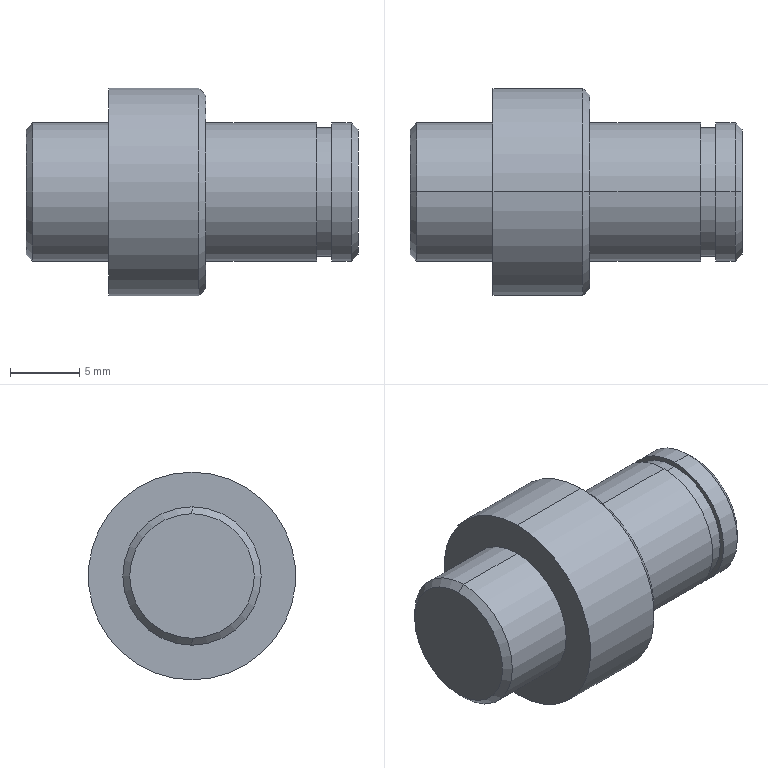Part | SolidWorks | features ICE 4, Chamfer 3, Extrusion 1, RefAxis 1 | 1 solid | 22 faces | box 24 x 15 x 15 mm | volume 2547 mm3 | cylinder 10 | cone 6 | plane 6 | commonest cylinder face diameters 10 x6 9.3 x2 15 x2
STEP:
#1=CARTESIAN_POINT('',(24.,0.,-4.5));
#2=VERTEX_POINT('',#1);
#3=CARTESIAN_POINT('',(24.,0.,4.5));
#4=VERTEX_POINT('',#3);
#5=CARTESIAN_POINT('',(24.,0.,0.));
#6=DIRECTION('',(1.,0.,0.));
#7=DIRECTION('',(0.,0.,-1.));
#8=AXIS2_PLACEMENT_3D('',#5,#6,#7);
#9=CIRCLE('',#8,4.5);
#10=EDGE_CURVE('',#2,#4,#9,.T.);
#11=ORIENTED_EDGE('',*,*,#10,.F.);
#12=CARTESIAN_POINT('',(23.5,0.,-5.));
#13=VERTEX_POINT('',#12);
#14=CARTESIAN_POINT('',(24.,0.,-4.5));
#15=DIRECTION('',(-0.7071,0.,-0.7071));
#16=VECTOR('',#15,1000.);
#17=LINE('',#14,#16);
#18=EDGE_CURVE('',#2,#13,#17,.T.);
#19=ORIENTED_EDGE('',*,*,#18,.T.);
#20=CARTESIAN_POINT('',(23.5,0.,5.));
#21=VERTEX_POINT('',#20);
#22=CARTESIAN_POINT('',(23.5,0.,0.));
#23=DIRECTION('',(-1.,0.,0.));
#24=DIRECTION('',(0.,0.,-1.));
#25=AXIS2_PLACEMENT_3D('',#22,#23,#24);
#26=CIRCLE('',#25,5.);
#27=EDGE_CURVE('',#21,#13,#26,.T.);
#28=ORIENTED_EDGE('',*,*,#27,.F.);
#29=CARTESIAN_POINT('',(24.,0.,4.5));
#30=DIRECTION('',(-0.7071,0.,0.7071));
#31=VECTOR('',#30,1000.);
#32=LINE('',#29,#31);
#33=EDGE_CURVE('',#4,#21,#32,.T.);
#34=ORIENTED_EDGE('',*,*,#33,.F.);
#35=EDGE_LOOP('',(#11,#19,#28,#34));
#36=FACE_OUTER_BOUND('',#35,.T.);
#37=CARTESIAN_POINT('',(24.,0.,0.));
#38=DIRECTION('',(-1.,0.,0.));
#39=DIRECTION('',(0.,0.,1.));
#40=AXIS2_PLACEMENT_3D('',#37,#38,#39);
#41=CONICAL_SURFACE('',#40,4.5,0.7854);
#42=ADVANCED_FACE('',(#36),#41,.T.);
#43=ORIENTED_EDGE('',*,*,#27,.T.);
#44=CARTESIAN_POINT('',(22.1,0.,-5.));
#45=VERTEX_POINT('',#44);
#46=CARTESIAN_POINT('',(24.,0.,-5.));
#47=DIRECTION('',(-1.,0.,0.));
#48=VECTOR('',#47,1000.);
#49=LINE('',#46,#48);
#50=EDGE_CURVE('',#13,#45,#49,.T.);
#51=ORIENTED_EDGE('',*,*,#50,.T.);
#52=CARTESIAN_POINT('',(22.1,0.,5.));
#53=VERTEX_POINT('',#52);
#54=CARTESIAN_POINT('',(22.1,0.,0.));
#55=DIRECTION('',(1.,0.,0.));
#56=DIRECTION('',(0.,0.,-1.));
#57=AXIS2_PLACEMENT_3D('',#54,#55,#56);
#58=CIRCLE('',#57,5.);
#59=EDGE_CURVE('',#45,#53,#58,.T.);
#60=ORIENTED_EDGE('',*,*,#59,.T.);
#61=CARTESIAN_POINT('',(24.,0.,5.));
#62=DIRECTION('',(-1.,0.,0.));
#63=VECTOR('',#62,1000.);
#64=LINE('',#61,#63);
#65=EDGE_CURVE('',#21,#53,#64,.T.);
#66=ORIENTED_EDGE('',*,*,#65,.F.);
#67=EDGE_LOOP('',(#43,#51,#60,#66));
#68=FACE_OUTER_BOUND('',#67,.T.);
#69=CARTESIAN_POINT('',(24.,0.,0.));
#70=DIRECTION('',(-1.,0.,0.));
#71=DIRECTION('',(0.,0.,1.));
#72=AXIS2_PLACEMENT_3D('',#69,#70,#71);
#73=CYLINDRICAL_SURFACE('',#72,5.);
#74=ADVANCED_FACE('',(#68),#73,.T.);
#75=CARTESIAN_POINT('',(22.1,0.,-4.65));
#76=VERTEX_POINT('',#75);
#77=CARTESIAN_POINT('',(22.1,0.,4.65));
#78=VERTEX_POINT('',#77);
#79=CARTESIAN_POINT('',(22.1,0.,0.));
#80=DIRECTION('',(1.,0.,0.));
#81=DIRECTION('',(0.,0.,-1.));
#82=AXIS2_PLACEMENT_3D('',#79,#80,#81);
#83=CIRCLE('',#82,4.65);
#84=EDGE_CURVE('',#76,#78,#83,.T.);
#85=ORIENTED_EDGE('',*,*,#84,.F.);
#86=CARTESIAN_POINT('',(21.,0.,-4.65));
#87=VERTEX_POINT('',#86);
#88=CARTESIAN_POINT('',(22.1,0.,-4.65));
#89=DIRECTION('',(-1.,0.,0.));
#90=VECTOR('',#89,1000.);
#91=LINE('',#88,#90);
#92=EDGE_CURVE('',#76,#87,#91,.T.);
#93=ORIENTED_EDGE('',*,*,#92,.T.);
#94=CARTESIAN_POINT('',(21.,0.,4.65));
#95=VERTEX_POINT('',#94);
#96=CARTESIAN_POINT('',(21.,0.,0.));
#97=DIRECTION('',(1.,0.,0.));
#98=DIRECTION('',(0.,0.,-1.));
#99=AXIS2_PLACEMENT_3D('',#96,#97,#98);
#100=CIRCLE('',#99,4.65);
#101=EDGE_CURVE('',#87,#95,#100,.T.);
#102=ORIENTED_EDGE('',*,*,#101,.T.);
#103=CARTESIAN_POINT('',(22.1,0.,4.65));
#104=DIRECTION('',(-1.,0.,0.));
#105=VECTOR('',#104,1000.);
#106=LINE('',#103,#105);
#107=EDGE_CURVE('',#78,#95,#106,.T.);
#108=ORIENTED_EDGE('',*,*,#107,.F.);
#109=EDGE_LOOP('',(#85,#93,#102,#108));
#110=FACE_OUTER_BOUND('',#109,.T.);
#111=CARTESIAN_POINT('',(22.1,0.,0.));
#112=DIRECTION('',(-1.,0.,0.));
#113=DIRECTION('',(0.,0.,1.));
#114=AXIS2_PLACEMENT_3D('',#111,#112,#113);
#115=CYLINDRICAL_SURFACE('',#114,4.65);
#116=ADVANCED_FACE('',(#110),#115,.T.);
#117=CARTESIAN_POINT('',(21.,0.,-5.));
#118=VERTEX_POINT('',#117);
#119=CARTESIAN_POINT('',(21.,0.,5.));
#120=VERTEX_POINT('',#119);
#121=CARTESIAN_POINT('',(21.,0.,0.));
#122=DIRECTION('',(1.,0.,0.));
#123=DIRECTION('',(0.,0.,-1.));
#124=AXIS2_PLACEMENT_3D('',#121,#122,#123);
#125=CIRCLE('',#124,5.);
#126=EDGE_CURVE('',#118,#120,#125,.T.);
#127=ORIENTED_EDGE('',*,*,#126,.F.);
#128=CARTESIAN_POINT('',(13.,0.,-5.));
#129=VERTEX_POINT('',#128);
#130=CARTESIAN_POINT('',(21.,0.,-5.));
#131=DIRECTION('',(-1.,0.,0.));
#132=VECTOR('',#131,1000.);
#133=LINE('',#130,#132);
#134=EDGE_CURVE('',#118,#129,#133,.T.);
#135=ORIENTED_EDGE('',*,*,#134,.T.);
#136=CARTESIAN_POINT('',(13.,0.,5.));
#137=VERTEX_POINT('',#136);
#138=CARTESIAN_POINT('',(13.,0.,0.));
#139=DIRECTION('',(1.,0.,0.));
#140=DIRECTION('',(0.,0.,-1.));
#141=AXIS2_PLACEMENT_3D('',#138,#139,#140);
#142=CIRCLE('',#141,5.);
#143=EDGE_CURVE('',#129,#137,#142,.T.);
#144=ORIENTED_EDGE('',*,*,#143,.T.);
#145=CARTESIAN_POINT('',(21.,0.,5.));
#146=DIRECTION('',(-1.,0.,0.));
#147=VECTOR('',#146,1000.);
#148=LINE('',#145,#147);
#149=EDGE_CURVE('',#120,#137,#148,.T.);
#150=ORIENTED_EDGE('',*,*,#149,.F.);
#151=EDGE_LOOP('',(#127,#135,#144,#150));
#152=FACE_OUTER_BOUND('',#151,.T.);
#153=CARTESIAN_POINT('',(21.,0.,0.));
#154=DIRECTION('',(-1.,0.,0.));
#155=DIRECTION('',(0.,0.,1.));
#156=AXIS2_PLACEMENT_3D('',#153,#154,#155);
#157=CYLINDRICAL_SURFACE('',#156,5.);
#158=ADVANCED_FACE('',(#152),#157,.T.);
#159=CARTESIAN_POINT('',(13.,0.,-7.));
#160=VERTEX_POINT('',#159);
#161=CARTESIAN_POINT('',(13.,0.,7.));
#162=VERTEX_POINT('',#161);
#163=CARTESIAN_POINT('',(13.,0.,0.));
#164=DIRECTION('',(1.,0.,0.));
#165=DIRECTION('',(0.,0.,-1.));
#166=AXIS2_PLACEMENT_3D('',#163,#164,#165);
#167=CIRCLE('',#166,7.);
#168=EDGE_CURVE('',#160,#162,#167,.T.);
#169=ORIENTED_EDGE('',*,*,#168,.F.);
#170=CARTESIAN_POINT('',(12.5,0.,-7.5));
#171=VERTEX_POINT('',#170);
#172=CARTESIAN_POINT('',(13.,0.,-7.));
#173=DIRECTION('',(-0.7071,0.,-0.7071));
#174=VECTOR('',#173,1000.);
#175=LINE('',#172,#174);
#176=EDGE_CURVE('',#160,#171,#175,.T.);
#177=ORIENTED_EDGE('',*,*,#176,.T.);
#178=CARTESIAN_POINT('',(12.5,0.,7.5));
#179=VERTEX_POINT('',#178);
#180=CARTESIAN_POINT('',(12.5,0.,0.));
#181=DIRECTION('',(-1.,0.,0.));
#182=DIRECTION('',(0.,0.,-1.));
#183=AXIS2_PLACEMENT_3D('',#180,#181,#182);
#184=CIRCLE('',#183,7.5);
#185=EDGE_CURVE('',#179,#171,#184,.T.);
#186=ORIENTED_EDGE('',*,*,#185,.F.);
#187=CARTESIAN_POINT('',(13.,0.,7.));
#188=DIRECTION('',(-0.7071,0.,0.7071));
#189=VECTOR('',#188,1000.);
#190=LINE('',#187,#189);
#191=EDGE_CURVE('',#162,#179,#190,.T.);
#192=ORIENTED_EDGE('',*,*,#191,.F.);
#193=EDGE_LOOP('',(#169,#177,#186,#192));
#194=FACE_OUTER_BOUND('',#193,.T.);
#195=CARTESIAN_POINT('',(13.,0.,0.));
#196=DIRECTION('',(-1.,0.,0.));
#197=DIRECTION('',(0.,0.,1.));
#198=AXIS2_PLACEMENT_3D('',#195,#196,#197);
#199=CONICAL_SURFACE('',#198,7.,0.7854);
#200=ADVANCED_FACE('',(#194),#199,.T.);
#201=ORIENTED_EDGE('',*,*,#185,.T.);
#202=CARTESIAN_POINT('',(6.,0.,-7.5));
#203=VERTEX_POINT('',#202);
#204=CARTESIAN_POINT('',(13.,0.,-7.5));
#205=DIRECTION('',(-1.,0.,0.));
#206=VECTOR('',#205,1000.);
#207=LINE('',#204,#206);
#208=EDGE_CURVE('',#171,#203,#207,.T.);
#209=ORIENTED_EDGE('',*,*,#208,.T.);
#210=CARTESIAN_POINT('',(6.,0.,7.5));
#211=VERTEX_POINT('',#210);
#212=CARTESIAN_POINT('',(6.,0.,0.));
#213=DIRECTION('',(1.,0.,0.));
#214=DIRECTION('',(0.,0.,-1.));
#215=AXIS2_PLACEMENT_3D('',#212,#213,#214);
#216=CIRCLE('',#215,7.5);
#217=EDGE_CURVE('',#203,#211,#216,.T.);
#218=ORIENTED_EDGE('',*,*,#217,.T.);
#219=CARTESIAN_POINT('',(13.,0.,7.5));
#220=DIRECTION('',(-1.,0.,0.));
#221=VECTOR('',#220,1000.);
#222=LINE('',#219,#221);
#223=EDGE_CURVE('',#179,#211,#222,.T.);
#224=ORIENTED_EDGE('',*,*,#223,.F.);
#225=EDGE_LOOP('',(#201,#209,#218,#224));
#226=FACE_OUTER_BOUND('',#225,.T.);
#227=CARTESIAN_POINT('',(13.,0.,0.));
#228=DIRECTION('',(-1.,0.,0.));
#229=DIRECTION('',(0.,0.,1.));
#230=AXIS2_PLACEMENT_3D('',#227,#228,#229);
#231=CYLINDRICAL_SURFACE('',#230,7.5);
#232=ADVANCED_FACE('',(#226),#231,.T.);
#233=CARTESIAN_POINT('',(0.,0.,4.5));
#234=VERTEX_POINT('',#233);
#235=CARTESIAN_POINT('',(0.,0.,-4.5));
#236=VERTEX_POINT('',#235);
#237=CARTESIAN_POINT('',(0.,0.,0.));
#238=DIRECTION('',(-1.,0.,0.));
#239=DIRECTION('',(0.,0.,-1.));
#240=AXIS2_PLACEMENT_3D('',#237,#238,#239);
#241=CIRCLE('',#240,4.5);
#242=EDGE_CURVE('',#234,#236,#241,.T.);
#243=ORIENTED_EDGE('',*,*,#242,.F.);
#244=CARTESIAN_POINT('',(0.5,0.,5.));
#245=VERTEX_POINT('',#244);
#246=CARTESIAN_POINT('',(0.5,0.,5.));
#247=DIRECTION('',(0.7071,0.,0.7071));
#248=VECTOR('',#247,1000.);
#249=LINE('',#246,#248);
#250=EDGE_CURVE('',#234,#245,#249,.T.);
#251=ORIENTED_EDGE('',*,*,#250,.T.);
#252=CARTESIAN_POINT('',(0.5,0.,-5.));
#253=VERTEX_POINT('',#252);
#254=CARTESIAN_POINT('',(0.5,0.,0.));
#255=DIRECTION('',(1.,0.,0.));
#256=DIRECTION('',(0.,0.,-1.));
#257=AXIS2_PLACEMENT_3D('',#254,#255,#256);
#258=CIRCLE('',#257,5.);
#259=EDGE_CURVE('',#253,#245,#258,.T.);
#260=ORIENTED_EDGE('',*,*,#259,.F.);
#261=CARTESIAN_POINT('',(0.5,0.,-5.));
#262=DIRECTION('',(0.7071,0.,-0.7071));
#263=VECTOR('',#262,1000.);
#264=LINE('',#261,#263);
#265=EDGE_CURVE('',#236,#253,#264,.T.);
#266=ORIENTED_EDGE('',*,*,#265,.F.);
#267=EDGE_LOOP('',(#243,#251,#260,#266));
#268=FACE_OUTER_BOUND('',#267,.T.);
#269=CARTESIAN_POINT('',(0.5,0.,0.));
#270=DIRECTION('',(1.,0.,0.));
#271=DIRECTION('',(0.,0.,-1.));
#272=AXIS2_PLACEMENT_3D('',#269,#270,#271);
#273=CONICAL_SURFACE('',#272,5.,0.7854);
#274=ADVANCED_FACE('',(#268),#273,.T.);
#275=CARTESIAN_POINT('',(6.,0.,-5.));
#276=VERTEX_POINT('',#275);
#277=CARTESIAN_POINT('',(6.,0.,5.));
#278=VERTEX_POINT('',#277);
#279=CARTESIAN_POINT('',(6.,0.,0.));
#280=DIRECTION('',(1.,0.,0.));
#281=DIRECTION('',(0.,0.,-1.));
#282=AXIS2_PLACEMENT_3D('',#279,#280,#281);
#283=CIRCLE('',#282,5.);
#284=EDGE_CURVE('',#276,#278,#283,.T.);
#285=ORIENTED_EDGE('',*,*,#284,.F.);
#286=CARTESIAN_POINT('',(6.,0.,-5.));
#287=DIRECTION('',(-1.,0.,0.));
#288=VECTOR('',#287,1000.);
#289=LINE('',#286,#288);
#290=EDGE_CURVE('',#276,#253,#289,.T.);
#291=ORIENTED_EDGE('',*,*,#290,.T.);
#292=ORIENTED_EDGE('',*,*,#259,.T.);
#293=CARTESIAN_POINT('',(6.,0.,5.));
#294=DIRECTION('',(-1.,0.,0.));
#295=VECTOR('',#294,1000.);
#296=LINE('',#293,#295);
#297=EDGE_CURVE('',#278,#245,#296,.T.);
#298=ORIENTED_EDGE('',*,*,#297,.F.);
#299=EDGE_LOOP('',(#285,#291,#292,#298));
#300=FACE_OUTER_BOUND('',#299,.T.);
#301=CARTESIAN_POINT('',(6.,0.,0.));
#302=DIRECTION('',(-1.,0.,0.));
#303=DIRECTION('',(0.,0.,1.));
#304=AXIS2_PLACEMENT_3D('',#301,#302,#303);
#305=CYLINDRICAL_SURFACE('',#304,5.);
#306=ADVANCED_FACE('',(#300),#305,.T.);
#307=ORIENTED_EDGE('',*,*,#290,.F.);
#308=CARTESIAN_POINT('',(6.,0.,0.));
#309=DIRECTION('',(1.,0.,0.));
#310=DIRECTION('',(0.,0.,-1.));
#311=AXIS2_PLACEMENT_3D('',#308,#309,#310);
#312=CIRCLE('',#311,5.);
#313=EDGE_CURVE('',#278,#276,#312,.T.);
#314=ORIENTED_EDGE('',*,*,#313,.F.);
#315=ORIENTED_EDGE('',*,*,#297,.T.);
#316=CARTESIAN_POINT('',(0.5,0.,0.));
#317=DIRECTION('',(1.,0.,0.));
#318=DIRECTION('',(0.,0.,-1.));
#319=AXIS2_PLACEMENT_3D('',#316,#317,#318);
#320=CIRCLE('',#319,5.);
#321=EDGE_CURVE('',#245,#253,#320,.T.);
#322=ORIENTED_EDGE('',*,*,#321,.T.);
#323=EDGE_LOOP('',(#307,#314,#315,#322));
#324=FACE_OUTER_BOUND('',#323,.T.);
#325=CARTESIAN_POINT('',(6.,0.,0.));
#326=DIRECTION('',(-1.,0.,0.));
#327=DIRECTION('',(0.,0.,1.));
#328=AXIS2_PLACEMENT_3D('',#325,#326,#327);
#329=CYLINDRICAL_SURFACE('',#328,5.);
#330=ADVANCED_FACE('',(#324),#329,.T.);
#331=CARTESIAN_POINT('',(0.,0.,0.));
#332=DIRECTION('',(-1.,0.,0.));
#333=DIRECTION('',(0.,0.,-1.));
#334=AXIS2_PLACEMENT_3D('',#331,#332,#333);
#335=CIRCLE('',#334,4.5);
#336=EDGE_CURVE('',#236,#234,#335,.T.);
#337=ORIENTED_EDGE('',*,*,#336,.T.);
#338=ORIENTED_EDGE('',*,*,#242,.T.);
#339=EDGE_LOOP('',(#337,#338));
#340=FACE_OUTER_BOUND('',#339,.T.);
#341=CARTESIAN_POINT('',(0.,0.,0.));
#342=DIRECTION('',(1.,0.,0.));
#343=DIRECTION('',(0.,0.,-1.));
#344=AXIS2_PLACEMENT_3D('',#341,#342,#343);
#345=PLANE('',#344);
#346=ADVANCED_FACE('',(#340),#345,.F.);
#347=ORIENTED_EDGE('',*,*,#250,.F.);
#348=ORIENTED_EDGE('',*,*,#336,.F.);
#349=ORIENTED_EDGE('',*,*,#265,.T.);
#350=ORIENTED_EDGE('',*,*,#321,.F.);
#351=EDGE_LOOP('',(#347,#348,#349,#350));
#352=FACE_OUTER_BOUND('',#351,.T.);
#353=CARTESIAN_POINT('',(0.5,0.,0.));
#354=DIRECTION('',(1.,0.,0.));
#355=DIRECTION('',(0.,0.,-1.));
#356=AXIS2_PLACEMENT_3D('',#353,#354,#355);
#357=CONICAL_SURFACE('',#356,5.,0.7854);
#358=ADVANCED_FACE('',(#352),#357,.T.);
#359=ORIENTED_EDGE('',*,*,#208,.F.);
#360=CARTESIAN_POINT('',(12.5,0.,0.));
#361=DIRECTION('',(-1.,0.,0.));
#362=DIRECTION('',(0.,0.,-1.));
#363=AXIS2_PLACEMENT_3D('',#360,#361,#362);
#364=CIRCLE('',#363,7.5);
#365=EDGE_CURVE('',#171,#179,#364,.T.);
#366=ORIENTED_EDGE('',*,*,#365,.T.);
#367=ORIENTED_EDGE('',*,*,#223,.T.);
#368=CARTESIAN_POINT('',(6.,0.,0.));
#369=DIRECTION('',(1.,0.,0.));
#370=DIRECTION('',(0.,0.,-1.));
#371=AXIS2_PLACEMENT_3D('',#368,#369,#370);
#372=CIRCLE('',#371,7.5);
#373=EDGE_CURVE('',#211,#203,#372,.T.);
#374=ORIENTED_EDGE('',*,*,#373,.T.);
#375=EDGE_LOOP('',(#359,#366,#367,#374));
#376=FACE_OUTER_BOUND('',#375,.T.);
#377=CARTESIAN_POINT('',(13.,0.,0.));
#378=DIRECTION('',(-1.,0.,0.));
#379=DIRECTION('',(0.,0.,1.));
#380=AXIS2_PLACEMENT_3D('',#377,#378,#379);
#381=CYLINDRICAL_SURFACE('',#380,7.5);
#382=ADVANCED_FACE('',(#376),#381,.T.);
#383=CARTESIAN_POINT('',(13.,0.,0.));
#384=DIRECTION('',(1.,0.,0.));
#385=DIRECTION('',(0.,0.,-1.));
#386=AXIS2_PLACEMENT_3D('',#383,#384,#385);
#387=CIRCLE('',#386,5.);
#388=EDGE_CURVE('',#137,#129,#387,.T.);
#389=ORIENTED_EDGE('',*,*,#388,.F.);
#390=ORIENTED_EDGE('',*,*,#143,.F.);
#391=EDGE_LOOP('',(#389,#390));
#392=FACE_BOUND('',#391,.T.);
#393=CARTESIAN_POINT('',(13.,0.,0.));
#394=DIRECTION('',(1.,0.,0.));
#395=DIRECTION('',(0.,0.,-1.));
#396=AXIS2_PLACEMENT_3D('',#393,#394,#395);
#397=CIRCLE('',#396,7.);
#398=EDGE_CURVE('',#162,#160,#397,.T.);
#399=ORIENTED_EDGE('',*,*,#398,.T.);
#400=ORIENTED_EDGE('',*,*,#168,.T.);
#401=EDGE_LOOP('',(#399,#400));
#402=FACE_OUTER_BOUND('',#401,.T.);
#403=CARTESIAN_POINT('',(13.,0.,0.));
#404=DIRECTION('',(1.,0.,0.));
#405=DIRECTION('',(0.,0.,-1.));
#406=AXIS2_PLACEMENT_3D('',#403,#404,#405);
#407=PLANE('',#406);
#408=ADVANCED_FACE('',(#392,#402),#407,.T.);
#409=ORIENTED_EDGE('',*,*,#313,.T.);
#410=ORIENTED_EDGE('',*,*,#284,.T.);
#411=EDGE_LOOP('',(#409,#410));
#412=FACE_BOUND('',#411,.T.);
#413=ORIENTED_EDGE('',*,*,#373,.F.);
#414=ORIENTED_EDGE('',*,*,#217,.F.);
#415=EDGE_LOOP('',(#413,#414));
#416=FACE_OUTER_BOUND('',#415,.T.);
#417=CARTESIAN_POINT('',(6.,0.,0.));
#418=DIRECTION('',(1.,0.,0.));
#419=DIRECTION('',(0.,0.,-1.));
#420=AXIS2_PLACEMENT_3D('',#417,#418,#419);
#421=PLANE('',#420);
#422=ADVANCED_FACE('',(#412,#416),#421,.F.);
#423=ORIENTED_EDGE('',*,*,#176,.F.);
#424=ORIENTED_EDGE('',*,*,#398,.F.);
#425=ORIENTED_EDGE('',*,*,#191,.T.);
#426=ORIENTED_EDGE('',*,*,#365,.F.);
#427=EDGE_LOOP('',(#423,#424,#425,#426));
#428=FACE_OUTER_BOUND('',#427,.T.);
#429=CARTESIAN_POINT('',(13.,0.,0.));
#430=DIRECTION('',(-1.,0.,0.));
#431=DIRECTION('',(0.,0.,1.));
#432=AXIS2_PLACEMENT_3D('',#429,#430,#431);
#433=CONICAL_SURFACE('',#432,7.,0.7854);
#434=ADVANCED_FACE('',(#428),#433,.T.);
#435=ORIENTED_EDGE('',*,*,#134,.F.);
#436=CARTESIAN_POINT('',(21.,0.,0.));
#437=DIRECTION('',(1.,0.,0.));
#438=DIRECTION('',(0.,0.,-1.));
#439=AXIS2_PLACEMENT_3D('',#436,#437,#438);
#440=CIRCLE('',#439,5.);
#441=EDGE_CURVE('',#120,#118,#440,.T.);
#442=ORIENTED_EDGE('',*,*,#441,.F.);
#443=ORIENTED_EDGE('',*,*,#149,.T.);
#444=ORIENTED_EDGE('',*,*,#388,.T.);
#445=EDGE_LOOP('',(#435,#442,#443,#444));
#446=FACE_OUTER_BOUND('',#445,.T.);
#447=CARTESIAN_POINT('',(21.,0.,0.));
#448=DIRECTION('',(-1.,0.,0.));
#449=DIRECTION('',(0.,0.,1.));
#450=AXIS2_PLACEMENT_3D('',#447,#448,#449);
#451=CYLINDRICAL_SURFACE('',#450,5.);
#452=ADVANCED_FACE('',(#446),#451,.T.);
#453=CARTESIAN_POINT('',(21.,0.,0.));
#454=DIRECTION('',(1.,0.,0.));
#455=DIRECTION('',(0.,0.,-1.));
#456=AXIS2_PLACEMENT_3D('',#453,#454,#455);
#457=CIRCLE('',#456,4.65);
#458=EDGE_CURVE('',#95,#87,#457,.T.);
#459=ORIENTED_EDGE('',*,*,#458,.F.);
#460=ORIENTED_EDGE('',*,*,#101,.F.);
#461=EDGE_LOOP('',(#459,#460));
#462=FACE_BOUND('',#461,.T.);
#463=ORIENTED_EDGE('',*,*,#441,.T.);
#464=ORIENTED_EDGE('',*,*,#126,.T.);
#465=EDGE_LOOP('',(#463,#464));
#466=FACE_OUTER_BOUND('',#465,.T.);
#467=CARTESIAN_POINT('',(21.,0.,0.));
#468=DIRECTION('',(1.,0.,0.));
#469=DIRECTION('',(0.,0.,-1.));
#470=AXIS2_PLACEMENT_3D('',#467,#468,#469);
#471=PLANE('',#470);
#472=ADVANCED_FACE('',(#462,#466),#471,.T.);
#473=ORIENTED_EDGE('',*,*,#92,.F.);
#474=CARTESIAN_POINT('',(22.1,0.,0.));
#475=DIRECTION('',(1.,0.,0.));
#476=DIRECTION('',(0.,0.,-1.));
#477=AXIS2_PLACEMENT_3D('',#474,#475,#476);
#478=CIRCLE('',#477,4.65);
#479=EDGE_CURVE('',#78,#76,#478,.T.);
#480=ORIENTED_EDGE('',*,*,#479,.F.);
#481=ORIENTED_EDGE('',*,*,#107,.T.);
#482=ORIENTED_EDGE('',*,*,#458,.T.);
#483=EDGE_LOOP('',(#473,#480,#481,#482));
#484=FACE_OUTER_BOUND('',#483,.T.);
#485=CARTESIAN_POINT('',(22.1,0.,0.));
#486=DIRECTION('',(-1.,0.,0.));
#487=DIRECTION('',(0.,0.,1.));
#488=AXIS2_PLACEMENT_3D('',#485,#486,#487);
#489=CYLINDRICAL_SURFACE('',#488,4.65);
#490=ADVANCED_FACE('',(#484),#489,.T.);
#491=ORIENTED_EDGE('',*,*,#50,.F.);
#492=CARTESIAN_POINT('',(23.5,0.,0.));
#493=DIRECTION('',(-1.,0.,0.));
#494=DIRECTION('',(0.,0.,-1.));
#495=AXIS2_PLACEMENT_3D('',#492,#493,#494);
#496=CIRCLE('',#495,5.);
#497=EDGE_CURVE('',#13,#21,#496,.T.);
#498=ORIENTED_EDGE('',*,*,#497,.T.);
#499=ORIENTED_EDGE('',*,*,#65,.T.);
#500=CARTESIAN_POINT('',(22.1,0.,0.));
#501=DIRECTION('',(1.,0.,0.));
#502=DIRECTION('',(0.,0.,-1.));
#503=AXIS2_PLACEMENT_3D('',#500,#501,#502);
#504=CIRCLE('',#503,5.);
#505=EDGE_CURVE('',#53,#45,#504,.T.);
#506=ORIENTED_EDGE('',*,*,#505,.T.);
#507=EDGE_LOOP('',(#491,#498,#499,#506));
#508=FACE_OUTER_BOUND('',#507,.T.);
#509=CARTESIAN_POINT('',(24.,0.,0.));
#510=DIRECTION('',(-1.,0.,0.));
#511=DIRECTION('',(0.,0.,1.));
#512=AXIS2_PLACEMENT_3D('',#509,#510,#511);
#513=CYLINDRICAL_SURFACE('',#512,5.);
#514=ADVANCED_FACE('',(#508),#513,.T.);
#515=CARTESIAN_POINT('',(24.,0.,0.));
#516=DIRECTION('',(1.,0.,0.));
#517=DIRECTION('',(0.,0.,-1.));
#518=AXIS2_PLACEMENT_3D('',#515,#516,#517);
#519=CIRCLE('',#518,4.5);
#520=EDGE_CURVE('',#4,#2,#519,.T.);
#521=ORIENTED_EDGE('',*,*,#520,.T.);
#522=ORIENTED_EDGE('',*,*,#10,.T.);
#523=EDGE_LOOP('',(#521,#522));
#524=FACE_OUTER_BOUND('',#523,.T.);
#525=CARTESIAN_POINT('',(24.,0.,0.));
#526=DIRECTION('',(1.,0.,0.));
#527=DIRECTION('',(0.,0.,-1.));
#528=AXIS2_PLACEMENT_3D('',#525,#526,#527);
#529=PLANE('',#528);
#530=ADVANCED_FACE('',(#524),#529,.T.);
#531=ORIENTED_EDGE('',*,*,#479,.T.);
#532=ORIENTED_EDGE('',*,*,#84,.T.);
#533=EDGE_LOOP('',(#531,#532));
#534=FACE_BOUND('',#533,.T.);
#535=ORIENTED_EDGE('',*,*,#505,.F.);
#536=ORIENTED_EDGE('',*,*,#59,.F.);
#537=EDGE_LOOP('',(#535,#536));
#538=FACE_OUTER_BOUND('',#537,.T.);
#539=CARTESIAN_POINT('',(22.1,0.,0.));
#540=DIRECTION('',(1.,0.,0.));
#541=DIRECTION('',(0.,0.,-1.));
#542=AXIS2_PLACEMENT_3D('',#539,#540,#541);
#543=PLANE('',#542);
#544=ADVANCED_FACE('',(#534,#538),#543,.F.);
#545=ORIENTED_EDGE('',*,*,#18,.F.);
#546=ORIENTED_EDGE('',*,*,#520,.F.);
#547=ORIENTED_EDGE('',*,*,#33,.T.);
#548=ORIENTED_EDGE('',*,*,#497,.F.);
#549=EDGE_LOOP('',(#545,#546,#547,#548));
#550=FACE_OUTER_BOUND('',#549,.T.);
#551=CARTESIAN_POINT('',(24.,0.,0.));
#552=DIRECTION('',(-1.,0.,0.));
#553=DIRECTION('',(0.,0.,1.));
#554=AXIS2_PLACEMENT_3D('',#551,#552,#553);
#555=CONICAL_SURFACE('',#554,4.5,0.7854);
#556=ADVANCED_FACE('',(#550),#555,.T.);
#557=CLOSED_SHELL('',(#42,#74,#116,#158,#200,#232,#274,#306,#330,#346,#358,#382,#408,#422,#434,#452,#472,#490,#514,#530,#544,#556));
#558=MANIFOLD_SOLID_BREP('',#557);
#559=CARTESIAN_POINT('',(0.,0.,0.));
#560=DIRECTION('',(0.,0.,1.));
#561=DIRECTION('',(1.,0.,0.));
#562=AXIS2_PLACEMENT_3D('',#559,#560,#561);
#563=(LENGTH_UNIT()NAMED_UNIT(*)SI_UNIT(.MILLI.,.METRE.));
#564=UNCERTAINTY_MEASURE_WITH_UNIT(LENGTH_MEASURE(0.00001),#563,'','');
#565=(NAMED_UNIT(*)PLANE_ANGLE_UNIT()SI_UNIT($,.RADIAN.));
#566=(NAMED_UNIT(*)SI_UNIT($,.STERADIAN.)SOLID_ANGLE_UNIT());
#567=(GEOMETRIC_REPRESENTATION_CONTEXT(3)GLOBAL_UNCERTAINTY_ASSIGNED_CONTEXT((#564))GLOBAL_UNIT_ASSIGNED_CONTEXT((#563,#565,#566))REPRESENTATION_CONTEXT('',''));
#568=ADVANCED_BREP_SHAPE_REPRESENTATION('',(#558,#562),#567);